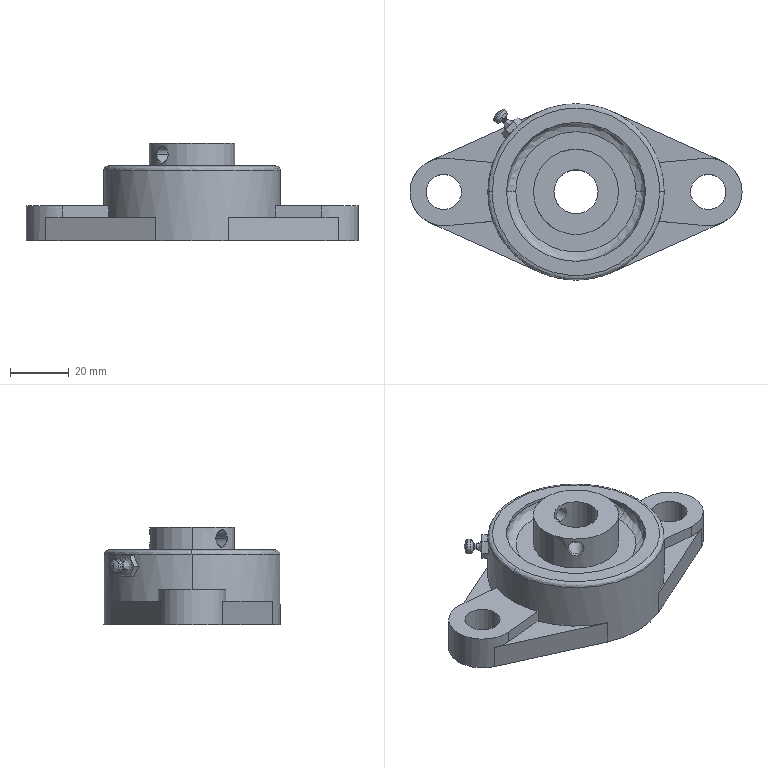Part | STEP file | 0228_Z_HDH151 | 1 solid | 82 faces | box 113 x 60 x 33.3 mm | volume 71474 mm3 | plane 30 | cylinder 27 | spline 18 | cone 7 | commonest cylinder face diameters 5.188 x4 12 x4 47.3 x4 23 x3 2 x2 5 x2